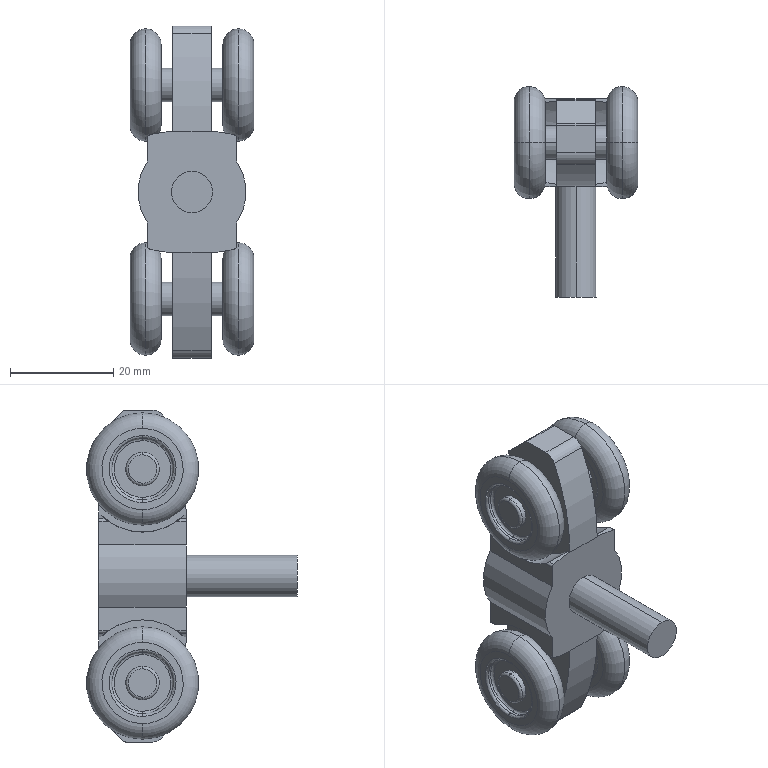Part | NX | features BREP 1 | 1 solid | 195 faces | box 24 x 40.9 x 64.4 mm | volume 18406 mm3 | cylinder 80 | torus 60 | plane 51 | cone 4 | commonest cylinder face diameters 1 x16 6.5 x16 12 x16 74.96 x8 23 x6 4 x4